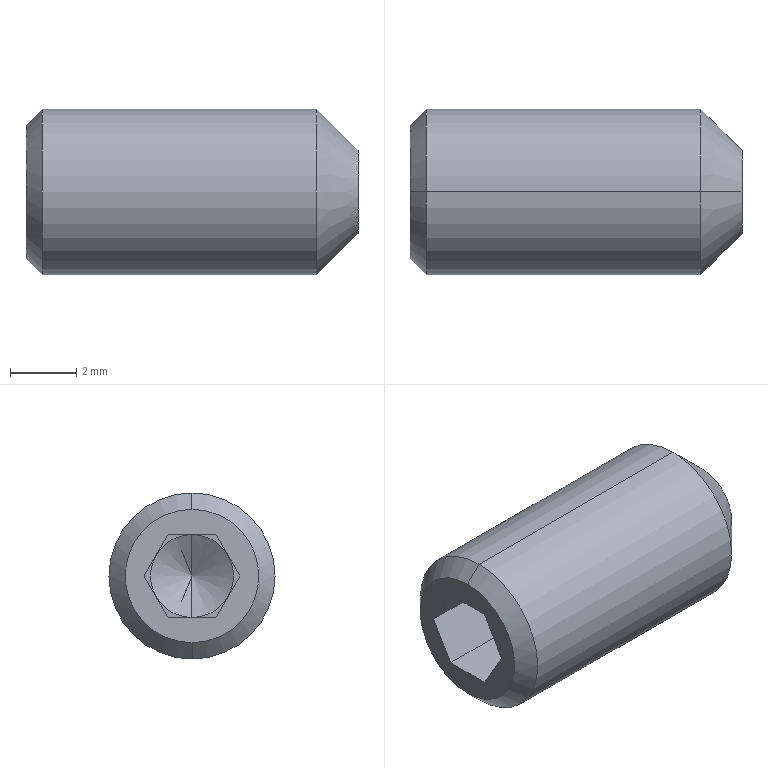Part | STEP file | 0230_301_MMSU5-10 | 1 solid | 23 faces | box 10 x 5 x 5 mm | volume 171.124 mm3 | plane 13 | cone 8 | cylinder 2 | commonest cylinder face diameters 5 x2
STEP:
#1=CARTESIAN_POINT('',(0.,0.,0.));
#2=DIRECTION('',(0.,0.,1.));
#3=DIRECTION('',(1.,0.,0.));
#4=AXIS2_PLACEMENT_3D('',#1,#2,#3);
#5=CARTESIAN_POINT('',(-4.51,0.,-2.5));
#6=VERTEX_POINT('',#5);
#7=CARTESIAN_POINT('',(-4.51,0.,2.5));
#8=VERTEX_POINT('',#7);
#9=CARTESIAN_POINT('',(-4.51,0.,0.));
#10=DIRECTION('',(1.,0.,0.));
#11=DIRECTION('',(0.,0.,-1.));
#12=AXIS2_PLACEMENT_3D('',#9,#10,#11);
#13=CIRCLE('',#12,2.5);
#14=CARTESIAN_POINT('',(-0.3797,0.,0.));
#15=DIRECTION('',(1.,0.,0.));
#16=DIRECTION('',(0.,0.,-1.));
#17=AXIS2_PLACEMENT_3D('',#14,#15,#16);
#18=CYLINDRICAL_SURFACE('',#17,2.5);
#19=CARTESIAN_POINT('',(0.,-4.13));
#20=DIRECTION('',(1.,0.));
#21=VECTOR('',#20,1.);
#22=LINE('',#19,#21);
#23=(GEOMETRIC_REPRESENTATION_CONTEXT(2)PARAMETRIC_REPRESENTATION_CONTEXT()REPRESENTATION_CONTEXT('',''));
#24=DEFINITIONAL_REPRESENTATION('',(#22),#23);
#25=PCURVE('',#18,#24);
#26=CARTESIAN_POINT('',(-4.51,0.,0.));
#27=DIRECTION('',(1.,0.,0.));
#28=DIRECTION('',(0.,0.,-1.));
#29=AXIS2_PLACEMENT_3D('',#26,#27,#28);
#30=CONICAL_SURFACE('',#29,2.5,0.7854);
#31=CARTESIAN_POINT('',(0.,0.));
#32=DIRECTION('',(1.,0.));
#33=VECTOR('',#32,1.);
#34=LINE('',#31,#33);
#35=(GEOMETRIC_REPRESENTATION_CONTEXT(2)PARAMETRIC_REPRESENTATION_CONTEXT()REPRESENTATION_CONTEXT('',''));
#36=DEFINITIONAL_REPRESENTATION('',(#34),#35);
#37=PCURVE('',#30,#36);
#38=SURFACE_CURVE('',#13,(#25,#37),.PCURVE_S1.);
#39=EDGE_CURVE('',#6,#8,#38,.T.);
#40=ORIENTED_EDGE('',*,*,#39,.T.);
#41=CARTESIAN_POINT('',(3.75,0.,2.5));
#42=VERTEX_POINT('',#41);
#43=CARTESIAN_POINT('',(-0.3797,0.,2.5));
#44=DIRECTION('',(1.,0.,0.));
#45=VECTOR('',#44,1.);
#46=LINE('',#43,#45);
#47=CARTESIAN_POINT('',(3.142,0.));
#48=DIRECTION('',(0.,1.));
#49=VECTOR('',#48,1.);
#50=LINE('',#47,#49);
#51=(GEOMETRIC_REPRESENTATION_CONTEXT(2)PARAMETRIC_REPRESENTATION_CONTEXT()REPRESENTATION_CONTEXT('',''));
#52=DEFINITIONAL_REPRESENTATION('',(#50),#51);
#53=PCURVE('',#18,#52);
#54=CARTESIAN_POINT('',(-0.3797,0.,0.));
#55=DIRECTION('',(1.,0.,0.));
#56=DIRECTION('',(0.,0.,-1.));
#57=AXIS2_PLACEMENT_3D('',#54,#55,#56);
#58=CYLINDRICAL_SURFACE('',#57,2.5);
#59=CARTESIAN_POINT('',(3.142,0.));
#60=DIRECTION('',(0.,1.));
#61=VECTOR('',#60,1.);
#62=LINE('',#59,#61);
#63=(GEOMETRIC_REPRESENTATION_CONTEXT(2)PARAMETRIC_REPRESENTATION_CONTEXT()REPRESENTATION_CONTEXT('',''));
#64=DEFINITIONAL_REPRESENTATION('',(#62),#63);
#65=PCURVE('',#58,#64);
#66=SURFACE_CURVE('',#46,(#53,#65),.PCURVE_S1.);
#67=EDGE_CURVE('',#8,#42,#66,.T.);
#68=ORIENTED_EDGE('',*,*,#67,.T.);
#69=CARTESIAN_POINT('',(3.75,0.,-2.5));
#70=VERTEX_POINT('',#69);
#71=CARTESIAN_POINT('',(3.75,0.,0.));
#72=DIRECTION('',(-1.,0.,0.));
#73=DIRECTION('',(0.,0.,-1.));
#74=AXIS2_PLACEMENT_3D('',#71,#72,#73);
#75=CIRCLE('',#74,2.5);
#76=CARTESIAN_POINT('',(6.283,4.13));
#77=DIRECTION('',(-1.,0.));
#78=VECTOR('',#77,1.);
#79=LINE('',#76,#78);
#80=(GEOMETRIC_REPRESENTATION_CONTEXT(2)PARAMETRIC_REPRESENTATION_CONTEXT()REPRESENTATION_CONTEXT('',''));
#81=DEFINITIONAL_REPRESENTATION('',(#79),#80);
#82=PCURVE('',#18,#81);
#83=CARTESIAN_POINT('',(3.75,0.,0.));
#84=DIRECTION('',(-1.,0.,0.));
#85=DIRECTION('',(0.,0.,1.));
#86=AXIS2_PLACEMENT_3D('',#83,#84,#85);
#87=CONICAL_SURFACE('',#86,2.5,0.7854);
#88=CARTESIAN_POINT('',(-3.142,0.));
#89=DIRECTION('',(1.,0.));
#90=VECTOR('',#89,1.);
#91=LINE('',#88,#90);
#92=(GEOMETRIC_REPRESENTATION_CONTEXT(2)PARAMETRIC_REPRESENTATION_CONTEXT()REPRESENTATION_CONTEXT('',''));
#93=DEFINITIONAL_REPRESENTATION('',(#91),#92);
#94=PCURVE('',#87,#93);
#95=SURFACE_CURVE('',#75,(#82,#94),.PCURVE_S1.);
#96=EDGE_CURVE('',#42,#70,#95,.T.);
#97=ORIENTED_EDGE('',*,*,#96,.T.);
#98=CARTESIAN_POINT('',(-0.3797,0.,-2.5));
#99=DIRECTION('',(1.,0.,0.));
#100=VECTOR('',#99,1.);
#101=LINE('',#98,#100);
#102=CARTESIAN_POINT('',(0.,0.));
#103=DIRECTION('',(0.,1.));
#104=VECTOR('',#103,1.);
#105=LINE('',#102,#104);
#106=(GEOMETRIC_REPRESENTATION_CONTEXT(2)PARAMETRIC_REPRESENTATION_CONTEXT()REPRESENTATION_CONTEXT('',''));
#107=DEFINITIONAL_REPRESENTATION('',(#105),#106);
#108=PCURVE('',#18,#107);
#109=CARTESIAN_POINT('',(6.283,0.));
#110=DIRECTION('',(0.,1.));
#111=VECTOR('',#110,1.);
#112=LINE('',#109,#111);
#113=(GEOMETRIC_REPRESENTATION_CONTEXT(2)PARAMETRIC_REPRESENTATION_CONTEXT()REPRESENTATION_CONTEXT('',''));
#114=DEFINITIONAL_REPRESENTATION('',(#112),#113);
#115=PCURVE('',#58,#114);
#116=SURFACE_CURVE('',#101,(#108,#115),.PCURVE_S1.);
#117=EDGE_CURVE('',#6,#70,#116,.T.);
#118=ORIENTED_EDGE('',*,*,#117,.F.);
#119=EDGE_LOOP('',(#40,#68,#97,#118));
#120=FACE_BOUND('',#119,.T.);
#121=ADVANCED_FACE('',(#120),#18,.T.);
#122=CARTESIAN_POINT('',(-5.,0.,-2.009));
#123=VERTEX_POINT('',#122);
#124=CARTESIAN_POINT('',(-5.,0.,2.009));
#125=VERTEX_POINT('',#124);
#126=CARTESIAN_POINT('',(-5.,0.,0.));
#127=DIRECTION('',(1.,0.,0.));
#128=DIRECTION('',(0.,0.,-1.));
#129=AXIS2_PLACEMENT_3D('',#126,#127,#128);
#130=CIRCLE('',#129,2.009);
#131=CARTESIAN_POINT('',(0.,-0.4905));
#132=DIRECTION('',(1.,0.));
#133=VECTOR('',#132,1.);
#134=LINE('',#131,#133);
#135=(GEOMETRIC_REPRESENTATION_CONTEXT(2)PARAMETRIC_REPRESENTATION_CONTEXT()REPRESENTATION_CONTEXT('',''));
#136=DEFINITIONAL_REPRESENTATION('',(#134),#135);
#137=PCURVE('',#30,#136);
#138=CARTESIAN_POINT('',(-5.,1.005,0.));
#139=DIRECTION('',(-1.,0.,0.));
#140=DIRECTION('',(0.,0.,1.));
#141=AXIS2_PLACEMENT_3D('',#138,#139,#140);
#142=PLANE('',#141);
#143=CARTESIAN_POINT('',(-2.009,-1.005));
#144=CARTESIAN_POINT('',(-2.009,2.476));
#145=CARTESIAN_POINT('',(1.005,0.7355));
#146=CARTESIAN_POINT('',(4.019,-1.005));
#147=CARTESIAN_POINT('',(1.005,-2.745));
#148=CARTESIAN_POINT('',(-2.009,-4.485));
#149=CARTESIAN_POINT('',(-2.009,-1.005));
#150=(BOUNDED_CURVE()B_SPLINE_CURVE(2,(#143,#144,#145,#146,#147,#148,#149),.UNSPECIFIED.,.T.,.F.)B_SPLINE_CURVE_WITH_KNOTS((1,2,2,2,2,1),(-2.094,0.,2.094,4.189,6.283,8.378),.UNSPECIFIED.)CURVE()GEOMETRIC_REPRESENTATION_ITEM()RATIONAL_B_SPLINE_CURVE((1.,0.5,1.,0.5,1.,0.5,1.))REPRESENTATION_ITEM(''));
#151=(GEOMETRIC_REPRESENTATION_CONTEXT(2)PARAMETRIC_REPRESENTATION_CONTEXT()REPRESENTATION_CONTEXT('',''));
#152=DEFINITIONAL_REPRESENTATION('',(#150),#151);
#153=PCURVE('',#142,#152);
#154=SURFACE_CURVE('',#130,(#137,#153),.PCURVE_S1.);
#155=EDGE_CURVE('',#123,#125,#154,.T.);
#156=ORIENTED_EDGE('',*,*,#155,.T.);
#157=CARTESIAN_POINT('',(-4.51,0.,2.5));
#158=DIRECTION('',(0.7071,0.,0.7071));
#159=VECTOR('',#158,1.);
#160=LINE('',#157,#159);
#161=CARTESIAN_POINT('',(3.142,0.));
#162=DIRECTION('',(0.,1.));
#163=VECTOR('',#162,1.);
#164=LINE('',#161,#163);
#165=(GEOMETRIC_REPRESENTATION_CONTEXT(2)PARAMETRIC_REPRESENTATION_CONTEXT()REPRESENTATION_CONTEXT('',''));
#166=DEFINITIONAL_REPRESENTATION('',(#164),#165);
#167=PCURVE('',#30,#166);
#168=CARTESIAN_POINT('',(-4.51,0.,0.));
#169=DIRECTION('',(1.,0.,0.));
#170=DIRECTION('',(0.,0.,-1.));
#171=AXIS2_PLACEMENT_3D('',#168,#169,#170);
#172=CONICAL_SURFACE('',#171,2.5,0.7854);
#173=CARTESIAN_POINT('',(3.142,0.));
#174=DIRECTION('',(0.,1.));
#175=VECTOR('',#174,1.);
#176=LINE('',#173,#175);
#177=(GEOMETRIC_REPRESENTATION_CONTEXT(2)PARAMETRIC_REPRESENTATION_CONTEXT()REPRESENTATION_CONTEXT('',''));
#178=DEFINITIONAL_REPRESENTATION('',(#176),#177);
#179=PCURVE('',#172,#178);
#180=SURFACE_CURVE('',#160,(#167,#179),.PCURVE_S1.);
#181=EDGE_CURVE('',#125,#8,#180,.T.);
#182=ORIENTED_EDGE('',*,*,#181,.T.);
#183=ORIENTED_EDGE('',*,*,#39,.F.);
#184=CARTESIAN_POINT('',(-4.51,0.,-2.5));
#185=DIRECTION('',(0.7071,0.,-0.7071));
#186=VECTOR('',#185,1.);
#187=LINE('',#184,#186);
#188=CARTESIAN_POINT('',(0.,0.));
#189=DIRECTION('',(0.,1.));
#190=VECTOR('',#189,1.);
#191=LINE('',#188,#190);
#192=(GEOMETRIC_REPRESENTATION_CONTEXT(2)PARAMETRIC_REPRESENTATION_CONTEXT()REPRESENTATION_CONTEXT('',''));
#193=DEFINITIONAL_REPRESENTATION('',(#191),#192);
#194=PCURVE('',#30,#193);
#195=CARTESIAN_POINT('',(6.283,0.));
#196=DIRECTION('',(0.,1.));
#197=VECTOR('',#196,1.);
#198=LINE('',#195,#197);
#199=(GEOMETRIC_REPRESENTATION_CONTEXT(2)PARAMETRIC_REPRESENTATION_CONTEXT()REPRESENTATION_CONTEXT('',''));
#200=DEFINITIONAL_REPRESENTATION('',(#198),#199);
#201=PCURVE('',#172,#200);
#202=SURFACE_CURVE('',#187,(#194,#201),.PCURVE_S1.);
#203=EDGE_CURVE('',#123,#6,#202,.T.);
#204=ORIENTED_EDGE('',*,*,#203,.F.);
#205=EDGE_LOOP('',(#156,#182,#183,#204));
#206=FACE_BOUND('',#205,.T.);
#207=ADVANCED_FACE('',(#206),#30,.T.);
#208=CARTESIAN_POINT('',(5.,0.,1.25));
#209=VERTEX_POINT('',#208);
#210=CARTESIAN_POINT('',(5.,0.,-1.25));
#211=VERTEX_POINT('',#210);
#212=CARTESIAN_POINT('',(5.,0.,0.));
#213=DIRECTION('',(-1.,0.,0.));
#214=DIRECTION('',(0.,1.,0.));
#215=AXIS2_PLACEMENT_3D('',#212,#213,#214);
#216=CIRCLE('',#215,1.25);
#217=CARTESIAN_POINT('',(-4.712,-1.25));
#218=DIRECTION('',(1.,0.));
#219=VECTOR('',#218,1.);
#220=LINE('',#217,#219);
#221=(GEOMETRIC_REPRESENTATION_CONTEXT(2)PARAMETRIC_REPRESENTATION_CONTEXT()REPRESENTATION_CONTEXT('',''));
#222=DEFINITIONAL_REPRESENTATION('',(#220),#221);
#223=PCURVE('',#87,#222);
#224=CARTESIAN_POINT('',(5.,0.,0.));
#225=DIRECTION('',(1.,0.,0.));
#226=DIRECTION('',(0.,0.,-1.));
#227=AXIS2_PLACEMENT_3D('',#224,#225,#226);
#228=CONICAL_SURFACE('',#227,1.25,1.03);
#229=CARTESIAN_POINT('',(7.854,0.));
#230=DIRECTION('',(-1.,0.));
#231=VECTOR('',#230,1.);
#232=LINE('',#229,#231);
#233=(GEOMETRIC_REPRESENTATION_CONTEXT(2)PARAMETRIC_REPRESENTATION_CONTEXT()REPRESENTATION_CONTEXT('',''));
#234=DEFINITIONAL_REPRESENTATION('',(#232),#233);
#235=PCURVE('',#228,#234);
#236=SURFACE_CURVE('',#216,(#223,#235),.PCURVE_S1.);
#237=EDGE_CURVE('',#209,#211,#236,.T.);
#238=ORIENTED_EDGE('',*,*,#237,.T.);
#239=CARTESIAN_POINT('',(3.75,0.,-2.5));
#240=DIRECTION('',(-0.7071,0.,-0.7071));
#241=VECTOR('',#240,1.);
#242=LINE('',#239,#241);
#243=CARTESIAN_POINT('',(3.142,0.));
#244=DIRECTION('',(0.,1.));
#245=VECTOR('',#244,1.);
#246=LINE('',#243,#245);
#247=(GEOMETRIC_REPRESENTATION_CONTEXT(2)PARAMETRIC_REPRESENTATION_CONTEXT()REPRESENTATION_CONTEXT('',''));
#248=DEFINITIONAL_REPRESENTATION('',(#246),#247);
#249=PCURVE('',#87,#248);
#250=CARTESIAN_POINT('',(3.75,0.,0.));
#251=DIRECTION('',(-1.,0.,0.));
#252=DIRECTION('',(0.,0.,1.));
#253=AXIS2_PLACEMENT_3D('',#250,#251,#252);
#254=CONICAL_SURFACE('',#253,2.5,0.7854);
#255=CARTESIAN_POINT('',(3.142,0.));
#256=DIRECTION('',(0.,1.));
#257=VECTOR('',#256,1.);
#258=LINE('',#255,#257);
#259=(GEOMETRIC_REPRESENTATION_CONTEXT(2)PARAMETRIC_REPRESENTATION_CONTEXT()REPRESENTATION_CONTEXT('',''));
#260=DEFINITIONAL_REPRESENTATION('',(#258),#259);
#261=PCURVE('',#254,#260);
#262=SURFACE_CURVE('',#242,(#249,#261),.PCURVE_S1.);
#263=EDGE_CURVE('',#211,#70,#262,.T.);
#264=ORIENTED_EDGE('',*,*,#263,.T.);
#265=ORIENTED_EDGE('',*,*,#96,.F.);
#266=CARTESIAN_POINT('',(3.75,0.,2.5));
#267=DIRECTION('',(-0.7071,0.,0.7071));
#268=VECTOR('',#267,1.);
#269=LINE('',#266,#268);
#270=CARTESIAN_POINT('',(0.,0.));
#271=DIRECTION('',(0.,1.));
#272=VECTOR('',#271,1.);
#273=LINE('',#270,#272);
#274=(GEOMETRIC_REPRESENTATION_CONTEXT(2)PARAMETRIC_REPRESENTATION_CONTEXT()REPRESENTATION_CONTEXT('',''));
#275=DEFINITIONAL_REPRESENTATION('',(#273),#274);
#276=PCURVE('',#87,#275);
#277=CARTESIAN_POINT('',(6.283,0.));
#278=DIRECTION('',(0.,1.));
#279=VECTOR('',#278,1.);
#280=LINE('',#277,#279);
#281=(GEOMETRIC_REPRESENTATION_CONTEXT(2)PARAMETRIC_REPRESENTATION_CONTEXT()REPRESENTATION_CONTEXT('',''));
#282=DEFINITIONAL_REPRESENTATION('',(#280),#281);
#283=PCURVE('',#254,#282);
#284=SURFACE_CURVE('',#269,(#276,#283),.PCURVE_S1.);
#285=EDGE_CURVE('',#209,#42,#284,.T.);
#286=ORIENTED_EDGE('',*,*,#285,.F.);
#287=EDGE_LOOP('',(#238,#264,#265,#286));
#288=FACE_BOUND('',#287,.T.);
#289=ADVANCED_FACE('',(#288),#87,.T.);
#290=CARTESIAN_POINT('',(5.,0.,0.));
#291=DIRECTION('',(-1.,0.,0.));
#292=DIRECTION('',(0.,1.,0.));
#293=AXIS2_PLACEMENT_3D('',#290,#291,#292);
#294=CIRCLE('',#293,1.25);
#295=CARTESIAN_POINT('',(5.,0.,0.));
#296=DIRECTION('',(1.,0.,0.));
#297=DIRECTION('',(0.,0.,-1.));
#298=AXIS2_PLACEMENT_3D('',#295,#296,#297);
#299=CONICAL_SURFACE('',#298,1.25,1.03);
#300=CARTESIAN_POINT('',(7.854,0.));
#301=DIRECTION('',(-1.,0.));
#302=VECTOR('',#301,1.);
#303=LINE('',#300,#302);
#304=(GEOMETRIC_REPRESENTATION_CONTEXT(2)PARAMETRIC_REPRESENTATION_CONTEXT()REPRESENTATION_CONTEXT('',''));
#305=DEFINITIONAL_REPRESENTATION('',(#303),#304);
#306=PCURVE('',#299,#305);
#307=CARTESIAN_POINT('',(1.571,-1.25));
#308=DIRECTION('',(1.,0.));
#309=VECTOR('',#308,1.);
#310=LINE('',#307,#309);
#311=(GEOMETRIC_REPRESENTATION_CONTEXT(2)PARAMETRIC_REPRESENTATION_CONTEXT()REPRESENTATION_CONTEXT('',''));
#312=DEFINITIONAL_REPRESENTATION('',(#310),#311);
#313=PCURVE('',#254,#312);
#314=SURFACE_CURVE('',#294,(#306,#313),.PCURVE_S1.);
#315=EDGE_CURVE('',#211,#209,#314,.T.);
#316=ORIENTED_EDGE('',*,*,#315,.T.);
#317=CARTESIAN_POINT('',(4.25,0.,0.));
#318=VERTEX_POINT('',#317);
#319=CARTESIAN_POINT('',(5.,0.,1.25));
#320=DIRECTION('',(0.5145,0.,0.8575));
#321=VECTOR('',#320,1.);
#322=LINE('',#319,#321);
#323=CARTESIAN_POINT('',(3.142,0.));
#324=DIRECTION('',(0.,1.));
#325=VECTOR('',#324,1.);
#326=LINE('',#323,#325);
#327=(GEOMETRIC_REPRESENTATION_CONTEXT(2)PARAMETRIC_REPRESENTATION_CONTEXT()REPRESENTATION_CONTEXT('',''));
#328=DEFINITIONAL_REPRESENTATION('',(#326),#327);
#329=PCURVE('',#299,#328);
#330=CARTESIAN_POINT('',(3.142,0.));
#331=DIRECTION('',(0.,1.));
#332=VECTOR('',#331,1.);
#333=LINE('',#330,#332);
#334=(GEOMETRIC_REPRESENTATION_CONTEXT(2)PARAMETRIC_REPRESENTATION_CONTEXT()REPRESENTATION_CONTEXT('',''));
#335=DEFINITIONAL_REPRESENTATION('',(#333),#334);
#336=PCURVE('',#228,#335);
#337=SURFACE_CURVE('',#322,(#329,#336),.PCURVE_S1.);
#338=EDGE_CURVE('',#318,#209,#337,.T.);
#339=ORIENTED_EDGE('',*,*,#338,.F.);
#340=CARTESIAN_POINT('',(5.,0.,-1.25));
#341=DIRECTION('',(0.5145,0.,-0.8575));
#342=VECTOR('',#341,1.);
#343=LINE('',#340,#342);
#344=CARTESIAN_POINT('',(6.283,0.));
#345=DIRECTION('',(0.,1.));
#346=VECTOR('',#345,1.);
#347=LINE('',#344,#346);
#348=(GEOMETRIC_REPRESENTATION_CONTEXT(2)PARAMETRIC_REPRESENTATION_CONTEXT()REPRESENTATION_CONTEXT('',''));
#349=DEFINITIONAL_REPRESENTATION('',(#347),#348);
#350=PCURVE('',#299,#349);
#351=CARTESIAN_POINT('',(0.,0.));
#352=DIRECTION('',(0.,1.));
#353=VECTOR('',#352,1.);
#354=LINE('',#351,#353);
#355=(GEOMETRIC_REPRESENTATION_CONTEXT(2)PARAMETRIC_REPRESENTATION_CONTEXT()REPRESENTATION_CONTEXT('',''));
#356=DEFINITIONAL_REPRESENTATION('',(#354),#355);
#357=PCURVE('',#228,#356);
#358=SURFACE_CURVE('',#343,(#350,#357),.PCURVE_S1.);
#359=EDGE_CURVE('',#318,#211,#358,.T.);
#360=ORIENTED_EDGE('',*,*,#359,.T.);
#361=EDGE_LOOP('',(#316,#339,#360));
#362=FACE_BOUND('',#361,.F.);
#363=ADVANCED_FACE('',(#362),#299,.F.);
#364=CARTESIAN_POINT('',(-3.,0.,1.25));
#365=VERTEX_POINT('',#364);
#366=CARTESIAN_POINT('',(-3.,-1.083,0.625));
#367=VERTEX_POINT('',#366);
#368=CARTESIAN_POINT('',(-3.,0.,0.));
#369=DIRECTION('',(1.,0.,0.));
#370=DIRECTION('',(0.,0.,1.));
#371=AXIS2_PLACEMENT_3D('',#368,#369,#370);
#372=CIRCLE('',#371,1.25);
#373=CARTESIAN_POINT('',(-3.,0.,0.));
#374=DIRECTION('',(-1.,0.,0.));
#375=DIRECTION('',(0.,0.,1.));
#376=AXIS2_PLACEMENT_3D('',#373,#374,#375);
#377=CONICAL_SURFACE('',#376,1.25,1.047);
#378=CARTESIAN_POINT('',(6.283,0.));
#379=DIRECTION('',(-1.,0.));
#380=VECTOR('',#379,1.);
#381=LINE('',#378,#380);
#382=(GEOMETRIC_REPRESENTATION_CONTEXT(2)PARAMETRIC_REPRESENTATION_CONTEXT()REPRESENTATION_CONTEXT('',''));
#383=DEFINITIONAL_REPRESENTATION('',(#381),#382);
#384=PCURVE('',#377,#383);
#385=CARTESIAN_POINT('',(-3.,0.,0.));
#386=DIRECTION('',(1.,0.,0.));
#387=DIRECTION('',(0.,0.,-1.));
#388=AXIS2_PLACEMENT_3D('',#385,#386,#387);
#389=PLANE('',#388);
#390=CARTESIAN_POINT('',(0.,0.));
#391=DIRECTION('',(-1.,0.));
#392=AXIS2_PLACEMENT_2D('',#390,#391);
#393=CIRCLE('',#392,1.25);
#394=(GEOMETRIC_REPRESENTATION_CONTEXT(2)PARAMETRIC_REPRESENTATION_CONTEXT()REPRESENTATION_CONTEXT('',''));
#395=DEFINITIONAL_REPRESENTATION('',(#393),#394);
#396=PCURVE('',#389,#395);
#397=SURFACE_CURVE('',#372,(#384,#396),.PCURVE_S1.);
#398=EDGE_CURVE('',#365,#367,#397,.T.);
#399=ORIENTED_EDGE('',*,*,#398,.T.);
#400=CARTESIAN_POINT('',(-3.,-1.083,-0.625));
#401=VERTEX_POINT('',#400);
#402=CARTESIAN_POINT('',(-3.,0.,0.));
#403=DIRECTION('',(1.,0.,0.));
#404=DIRECTION('',(0.,0.,1.));
#405=AXIS2_PLACEMENT_3D('',#402,#403,#404);
#406=CIRCLE('',#405,1.25);
#407=CARTESIAN_POINT('',(6.283,0.));
#408=DIRECTION('',(-1.,0.));
#409=VECTOR('',#408,1.);
#410=LINE('',#407,#409);
#411=(GEOMETRIC_REPRESENTATION_CONTEXT(2)PARAMETRIC_REPRESENTATION_CONTEXT()REPRESENTATION_CONTEXT('',''));
#412=DEFINITIONAL_REPRESENTATION('',(#410),#411);
#413=PCURVE('',#377,#412);
#414=CARTESIAN_POINT('',(-3.,0.,0.));
#415=DIRECTION('',(1.,0.,0.));
#416=DIRECTION('',(0.,0.,-1.));
#417=AXIS2_PLACEMENT_3D('',#414,#415,#416);
#418=PLANE('',#417);
#419=CARTESIAN_POINT('',(0.,0.));
#420=DIRECTION('',(-1.,0.));
#421=AXIS2_PLACEMENT_2D('',#419,#420);
#422=CIRCLE('',#421,1.25);
#423=(GEOMETRIC_REPRESENTATION_CONTEXT(2)PARAMETRIC_REPRESENTATION_CONTEXT()REPRESENTATION_CONTEXT('',''));
#424=DEFINITIONAL_REPRESENTATION('',(#422),#423);
#425=PCURVE('',#418,#424);
#426=SURFACE_CURVE('',#406,(#413,#425),.PCURVE_S1.);
#427=EDGE_CURVE('',#367,#401,#426,.T.);
#428=ORIENTED_EDGE('',*,*,#427,.T.);
#429=CARTESIAN_POINT('',(-3.,0.,-1.25));
#430=VERTEX_POINT('',#429);
#431=CARTESIAN_POINT('',(-3.,0.,0.));
#432=DIRECTION('',(-1.,0.,0.));
#433=DIRECTION('',(0.,0.,1.));
#434=AXIS2_PLACEMENT_3D('',#431,#432,#433);
#435=CIRCLE('',#434,1.25);
#436=CARTESIAN_POINT('',(0.,0.));
#437=DIRECTION('',(1.,0.));
#438=VECTOR('',#437,1.);
#439=LINE('',#436,#438);
#440=(GEOMETRIC_REPRESENTATION_CONTEXT(2)PARAMETRIC_REPRESENTATION_CONTEXT()REPRESENTATION_CONTEXT('',''));
#441=DEFINITIONAL_REPRESENTATION('',(#439),#440);
#442=PCURVE('',#377,#441);
#443=CARTESIAN_POINT('',(-3.,0.,0.));
#444=DIRECTION('',(1.,0.,0.));
#445=DIRECTION('',(0.,0.,-1.));
#446=AXIS2_PLACEMENT_3D('',#443,#444,#445);
#447=PLANE('',#446);
#448=CARTESIAN_POINT('',(-1.25,0.));
#449=CARTESIAN_POINT('',(-1.25,2.165));
#450=CARTESIAN_POINT('',(0.625,1.083));
#451=CARTESIAN_POINT('',(2.5,0.));
#452=CARTESIAN_POINT('',(0.625,-1.083));
#453=CARTESIAN_POINT('',(-1.25,-2.165));
#454=CARTESIAN_POINT('',(-1.25,0.));
#455=(BOUNDED_CURVE()B_SPLINE_CURVE(2,(#448,#449,#450,#451,#452,#453,#454),.UNSPECIFIED.,.T.,.F.)B_SPLINE_CURVE_WITH_KNOTS((1,2,2,2,2,1),(-2.094,0.,2.094,4.189,6.283,8.378),.UNSPECIFIED.)CURVE()GEOMETRIC_REPRESENTATION_ITEM()RATIONAL_B_SPLINE_CURVE((1.,0.5,1.,0.5,1.,0.5,1.))REPRESENTATION_ITEM(''));
#456=(GEOMETRIC_REPRESENTATION_CONTEXT(2)PARAMETRIC_REPRESENTATION_CONTEXT()REPRESENTATION_CONTEXT('',''));
#457=DEFINITIONAL_REPRESENTATION('',(#455),#456);
#458=PCURVE('',#447,#457);
#459=SURFACE_CURVE('',#435,(#442,#458),.PCURVE_S1.);
#460=EDGE_CURVE('',#430,#401,#459,.T.);
#461=ORIENTED_EDGE('',*,*,#460,.F.);
#462=CARTESIAN_POINT('',(-2.278,0.,0.));
#463=VERTEX_POINT('',#462);
#464=CARTESIAN_POINT('',(-3.,0.,-1.25));
#465=DIRECTION('',(-0.5,0.,-0.866));
#466=VECTOR('',#465,1.);
#467=LINE('',#464,#466);
#468=CARTESIAN_POINT('',(3.142,0.));
#469=DIRECTION('',(0.,1.));
#470=VECTOR('',#469,1.);
#471=LINE('',#468,#470);
#472=(GEOMETRIC_REPRESENTATION_CONTEXT(2)PARAMETRIC_REPRESENTATION_CONTEXT()REPRESENTATION_CONTEXT('',''));
#473=DEFINITIONAL_REPRESENTATION('',(#471),#472);
#474=PCURVE('',#377,#473);
#475=CARTESIAN_POINT('',(-3.,0.,0.));
#476=DIRECTION('',(-1.,0.,0.));
#477=DIRECTION('',(0.,0.,1.));
#478=AXIS2_PLACEMENT_3D('',#475,#476,#477);
#479=CONICAL_SURFACE('',#478,1.25,1.047);
#480=CARTESIAN_POINT('',(3.142,0.));
#481=DIRECTION('',(0.,1.));
#482=VECTOR('',#481,1.);
#483=LINE('',#480,#482);
#484=(GEOMETRIC_REPRESENTATION_CONTEXT(2)PARAMETRIC_REPRESENTATION_CONTEXT()REPRESENTATION_CONTEXT('',''));
#485=DEFINITIONAL_REPRESENTATION('',(#483),#484);
#486=PCURVE('',#479,#485);
#487=SURFACE_CURVE('',#467,(#474,#486),.PCURVE_S1.);
#488=EDGE_CURVE('',#463,#430,#487,.T.);
#489=ORIENTED_EDGE('',*,*,#488,.F.);
#490=CARTESIAN_POINT('',(-3.,0.,1.25));
#491=DIRECTION('',(-0.5,0.,0.866));
#492=VECTOR('',#491,1.);
#493=LINE('',#490,#492);
#494=CARTESIAN_POINT('',(6.283,0.));
#495=DIRECTION('',(0.,1.));
#496=VECTOR('',#495,1.);
#497=LINE('',#494,#496);
#498=(GEOMETRIC_REPRESENTATION_CONTEXT(2)PARAMETRIC_REPRESENTATION_CONTEXT()REPRESENTATION_CONTEXT('',''));
#499=DEFINITIONAL_REPRESENTATION('',(#497),#498);
#500=PCURVE('',#377,#499);
#501=CARTESIAN_POINT('',(0.,0.));
#502=DIRECTION('',(0.,1.));
#503=VECTOR('',#502,1.);
#504=LINE('',#501,#503);
#505=(GEOMETRIC_REPRESENTATION_CONTEXT(2)PARAMETRIC_REPRESENTATION_CONTEXT()REPRESENTATION_CONTEXT('',''));
#506=DEFINITIONAL_REPRESENTATION('',(#504),#505);
#507=PCURVE('',#479,#506);
#508=SURFACE_CURVE('',#493,(#500,#507),.PCURVE_S1.);
#509=EDGE_CURVE('',#463,#365,#508,.T.);
#510=ORIENTED_EDGE('',*,*,#509,.T.);
#511=EDGE_LOOP('',(#399,#428,#461,#489,#510));
#512=FACE_BOUND('',#511,.F.);
#513=ADVANCED_FACE('',(#512),#377,.F.);
#514=ORIENTED_EDGE('',*,*,#67,.F.);
#515=CARTESIAN_POINT('',(-4.51,0.,0.));
#516=DIRECTION('',(1.,0.,0.));
#517=DIRECTION('',(0.,0.,-1.));
#518=AXIS2_PLACEMENT_3D('',#515,#516,#517);
#519=CIRCLE('',#518,2.5);
#520=CARTESIAN_POINT('',(0.,-4.13));
#521=DIRECTION('',(1.,0.));
#522=VECTOR('',#521,1.);
#523=LINE('',#520,#522);
#524=(GEOMETRIC_REPRESENTATION_CONTEXT(2)PARAMETRIC_REPRESENTATION_CONTEXT()REPRESENTATION_CONTEXT('',''));
#525=DEFINITIONAL_REPRESENTATION('',(#523),#524);
#526=PCURVE('',#58,#525);
#527=CARTESIAN_POINT('',(0.,0.));
#528=DIRECTION('',(1.,0.));
#529=VECTOR('',#528,1.);
#530=LINE('',#527,#529);
#531=(GEOMETRIC_REPRESENTATION_CONTEXT(2)PARAMETRIC_REPRESENTATION_CONTEXT()REPRESENTATION_CONTEXT('',''));
#532=DEFINITIONAL_REPRESENTATION('',(#530),#531);
#533=PCURVE('',#172,#532);
#534=SURFACE_CURVE('',#519,(#526,#533),.PCURVE_S1.);
#535=EDGE_CURVE('',#8,#6,#534,.T.);
#536=ORIENTED_EDGE('',*,*,#535,.T.);
#537=ORIENTED_EDGE('',*,*,#117,.T.);
#538=CARTESIAN_POINT('',(3.75,0.,0.));
#539=DIRECTION('',(-1.,0.,0.));
#540=DIRECTION('',(0.,0.,-1.));
#541=AXIS2_PLACEMENT_3D('',#538,#539,#540);
#542=CIRCLE('',#541,2.5);
#543=CARTESIAN_POINT('',(6.283,4.13));
#544=DIRECTION('',(-1.,0.));
#545=VECTOR('',#544,1.);
#546=LINE('',#543,#545);
#547=(GEOMETRIC_REPRESENTATION_CONTEXT(2)PARAMETRIC_REPRESENTATION_CONTEXT()REPRESENTATION_CONTEXT('',''));
#548=DEFINITIONAL_REPRESENTATION('',(#546),#547);
#549=PCURVE('',#58,#548);
#550=CARTESIAN_POINT('',(3.142,0.));
#551=DIRECTION('',(1.,0.));
#552=VECTOR('',#551,1.);
#553=LINE('',#550,#552);
#554=(GEOMETRIC_REPRESENTATION_CONTEXT(2)PARAMETRIC_REPRESENTATION_CONTEXT()REPRESENTATION_CONTEXT('',''));
#555=DEFINITIONAL_REPRESENTATION('',(#553),#554);
#556=PCURVE('',#254,#555);
#557=SURFACE_CURVE('',#542,(#549,#556),.PCURVE_S1.);
#558=EDGE_CURVE('',#70,#42,#557,.T.);
#559=ORIENTED_EDGE('',*,*,#558,.T.);
#560=EDGE_LOOP('',(#514,#536,#537,#559));
#561=FACE_BOUND('',#560,.T.);
#562=ADVANCED_FACE('',(#561),#58,.T.);
#563=ORIENTED_EDGE('',*,*,#181,.F.);
#564=CARTESIAN_POINT('',(-5.,0.,0.));
#565=DIRECTION('',(1.,0.,0.));
#566=DIRECTION('',(0.,0.,-1.));
#567=AXIS2_PLACEMENT_3D('',#564,#565,#566);
#568=CIRCLE('',#567,2.009);
#569=CARTESIAN_POINT('',(0.,-0.4905));
#570=DIRECTION('',(1.,0.));
#571=VECTOR('',#570,1.);
#572=LINE('',#569,#571);
#573=(GEOMETRIC_REPRESENTATION_CONTEXT(2)PARAMETRIC_REPRESENTATION_CONTEXT()REPRESENTATION_CONTEXT('',''));
#574=DEFINITIONAL_REPRESENTATION('',(#572),#573);
#575=PCURVE('',#172,#574);
#576=CARTESIAN_POINT('',(-2.009,-1.005));
#577=CARTESIAN_POINT('',(-2.009,2.476));
#578=CARTESIAN_POINT('',(1.005,0.7355));
#579=CARTESIAN_POINT('',(4.019,-1.005));
#580=CARTESIAN_POINT('',(1.005,-2.745));
#581=CARTESIAN_POINT('',(-2.009,-4.485));
#582=CARTESIAN_POINT('',(-2.009,-1.005));
#583=(BOUNDED_CURVE()B_SPLINE_CURVE(2,(#576,#577,#578,#579,#580,#581,#582),.UNSPECIFIED.,.T.,.F.)B_SPLINE_CURVE_WITH_KNOTS((1,2,2,2,2,1),(-2.094,0.,2.094,4.189,6.283,8.378),.UNSPECIFIED.)CURVE()GEOMETRIC_REPRESENTATION_ITEM()RATIONAL_B_SPLINE_CURVE((1.,0.5,1.,0.5,1.,0.5,1.))REPRESENTATION_ITEM(''));
#584=(GEOMETRIC_REPRESENTATION_CONTEXT(2)PARAMETRIC_REPRESENTATION_CONTEXT()REPRESENTATION_CONTEXT('',''));
#585=DEFINITIONAL_REPRESENTATION('',(#583),#584);
#586=PCURVE('',#142,#585);
#587=SURFACE_CURVE('',#568,(#575,#586),.PCURVE_S1.);
#588=EDGE_CURVE('',#125,#123,#587,.T.);
#589=ORIENTED_EDGE('',*,*,#588,.T.);
#590=ORIENTED_EDGE('',*,*,#203,.T.);
#591=ORIENTED_EDGE('',*,*,#535,.F.);
#592=EDGE_LOOP('',(#563,#589,#590,#591));
#593=FACE_BOUND('',#592,.T.);
#594=ADVANCED_FACE('',(#593),#172,.T.);
#595=ORIENTED_EDGE('',*,*,#263,.F.);
#596=ORIENTED_EDGE('',*,*,#315,.T.);
#597=ORIENTED_EDGE('',*,*,#285,.T.);
#598=ORIENTED_EDGE('',*,*,#558,.F.);
#599=EDGE_LOOP('',(#595,#596,#597,#598));
#600=FACE_BOUND('',#599,.T.);
#601=ADVANCED_FACE('',(#600),#254,.T.);
#602=ORIENTED_EDGE('',*,*,#155,.F.);
#603=ORIENTED_EDGE('',*,*,#588,.F.);
#604=EDGE_LOOP('',(#602,#603));
#605=FACE_BOUND('',#604,.T.);
#606=CARTESIAN_POINT('',(-5.,-0.7217,-1.25));
#607=VERTEX_POINT('',#606);
#608=CARTESIAN_POINT('',(-5.,0.7217,-1.25));
#609=VERTEX_POINT('',#608);
#610=CARTESIAN_POINT('',(-5.,0.7217,-1.25));
#611=DIRECTION('',(0.,1.,0.));
#612=VECTOR('',#611,1.);
#613=LINE('',#610,#612);
#614=CARTESIAN_POINT('',(-1.25,-0.2831));
#615=DIRECTION('',(0.,1.));
#616=VECTOR('',#615,1.);
#617=LINE('',#614,#616);
#618=(GEOMETRIC_REPRESENTATION_CONTEXT(2)PARAMETRIC_REPRESENTATION_CONTEXT()REPRESENTATION_CONTEXT('',''));
#619=DEFINITIONAL_REPRESENTATION('',(#617),#618);
#620=PCURVE('',#142,#619);
#621=CARTESIAN_POINT('',(-5.,0.7217,-1.25));
#622=DIRECTION('',(0.,0.,-1.));
#623=DIRECTION('',(-1.,0.,0.));
#624=AXIS2_PLACEMENT_3D('',#621,#622,#623);
#625=PLANE('',#624);
#626=CARTESIAN_POINT('',(0.,0.));
#627=DIRECTION('',(0.,1.));
#628=VECTOR('',#627,1.);
#629=LINE('',#626,#628);
#630=(GEOMETRIC_REPRESENTATION_CONTEXT(2)PARAMETRIC_REPRESENTATION_CONTEXT()REPRESENTATION_CONTEXT('',''));
#631=DEFINITIONAL_REPRESENTATION('',(#629),#630);
#632=PCURVE('',#625,#631);
#633=SURFACE_CURVE('',#613,(#620,#632),.PCURVE_S1.);
#634=EDGE_CURVE('',#607,#609,#633,.T.);
#635=ORIENTED_EDGE('',*,*,#634,.T.);
#636=CARTESIAN_POINT('',(-5.,1.443,0.));
#637=VERTEX_POINT('',#636);
#638=CARTESIAN_POINT('',(-5.,0.7217,-1.25));
#639=DIRECTION('',(0.,0.5,0.866));
#640=VECTOR('',#639,1.);
#641=LINE('',#638,#640);
#642=CARTESIAN_POINT('',(-1.25,-0.2831));
#643=DIRECTION('',(0.866,0.5));
#644=VECTOR('',#643,1.);
#645=LINE('',#642,#644);
#646=(GEOMETRIC_REPRESENTATION_CONTEXT(2)PARAMETRIC_REPRESENTATION_CONTEXT()REPRESENTATION_CONTEXT('',''));
#647=DEFINITIONAL_REPRESENTATION('',(#645),#646);
#648=PCURVE('',#142,#647);
#649=CARTESIAN_POINT('',(-5.,1.443,0.));
#650=DIRECTION('',(0.,0.866,-0.5));
#651=DIRECTION('',(0.,0.5,0.866));
#652=AXIS2_PLACEMENT_3D('',#649,#650,#651);
#653=PLANE('',#652);
#654=CARTESIAN_POINT('',(-1.443,0.));
#655=DIRECTION('',(1.,0.));
#656=VECTOR('',#655,1.);
#657=LINE('',#654,#656);
#658=(GEOMETRIC_REPRESENTATION_CONTEXT(2)PARAMETRIC_REPRESENTATION_CONTEXT()REPRESENTATION_CONTEXT('',''));
#659=DEFINITIONAL_REPRESENTATION('',(#657),#658);
#660=PCURVE('',#653,#659);
#661=SURFACE_CURVE('',#641,(#648,#660),.PCURVE_S1.);
#662=EDGE_CURVE('',#609,#637,#661,.T.);
#663=ORIENTED_EDGE('',*,*,#662,.T.);
#664=CARTESIAN_POINT('',(-5.,0.7217,1.25));
#665=VERTEX_POINT('',#664);
#666=CARTESIAN_POINT('',(-5.,0.7217,1.25));
#667=DIRECTION('',(0.,-0.5,0.866));
#668=VECTOR('',#667,1.);
#669=LINE('',#666,#668);
#670=CARTESIAN_POINT('',(1.25,-0.2831));
#671=DIRECTION('',(0.866,-0.5));
#672=VECTOR('',#671,1.);
#673=LINE('',#670,#672);
#674=(GEOMETRIC_REPRESENTATION_CONTEXT(2)PARAMETRIC_REPRESENTATION_CONTEXT()REPRESENTATION_CONTEXT('',''));
#675=DEFINITIONAL_REPRESENTATION('',(#673),#674);
#676=PCURVE('',#142,#675);
#677=CARTESIAN_POINT('',(-5.,0.7217,1.25));
#678=DIRECTION('',(0.,0.866,0.5));
#679=DIRECTION('',(0.,-0.5,0.866));
#680=AXIS2_PLACEMENT_3D('',#677,#678,#679);
#681=PLANE('',#680);
#682=CARTESIAN_POINT('',(0.,0.));
#683=DIRECTION('',(1.,0.));
#684=VECTOR('',#683,1.);
#685=LINE('',#682,#684);
#686=(GEOMETRIC_REPRESENTATION_CONTEXT(2)PARAMETRIC_REPRESENTATION_CONTEXT()REPRESENTATION_CONTEXT('',''));
#687=DEFINITIONAL_REPRESENTATION('',(#685),#686);
#688=PCURVE('',#681,#687);
#689=SURFACE_CURVE('',#669,(#676,#688),.PCURVE_S1.);
#690=EDGE_CURVE('',#637,#665,#689,.T.);
#691=ORIENTED_EDGE('',*,*,#690,.T.);
#692=CARTESIAN_POINT('',(-5.,-0.7217,1.25));
#693=VERTEX_POINT('',#692);
#694=CARTESIAN_POINT('',(-5.,-0.7217,1.25));
#695=DIRECTION('',(0.,-1.,0.));
#696=VECTOR('',#695,1.);
#697=LINE('',#694,#696);
#698=CARTESIAN_POINT('',(1.25,-1.726));
#699=DIRECTION('',(0.,-1.));
#700=VECTOR('',#699,1.);
#701=LINE('',#698,#700);
#702=(GEOMETRIC_REPRESENTATION_CONTEXT(2)PARAMETRIC_REPRESENTATION_CONTEXT()REPRESENTATION_CONTEXT('',''));
#703=DEFINITIONAL_REPRESENTATION('',(#701),#702);
#704=PCURVE('',#142,#703);
#705=CARTESIAN_POINT('',(-5.,-0.7217,1.25));
#706=DIRECTION('',(0.,0.,1.));
#707=DIRECTION('',(1.,0.,0.));
#708=AXIS2_PLACEMENT_3D('',#705,#706,#707);
#709=PLANE('',#708);
#710=CARTESIAN_POINT('',(0.,0.));
#711=DIRECTION('',(0.,-1.));
#712=VECTOR('',#711,1.);
#713=LINE('',#710,#712);
#714=(GEOMETRIC_REPRESENTATION_CONTEXT(2)PARAMETRIC_REPRESENTATION_CONTEXT()REPRESENTATION_CONTEXT('',''));
#715=DEFINITIONAL_REPRESENTATION('',(#713),#714);
#716=PCURVE('',#709,#715);
#717=SURFACE_CURVE('',#697,(#704,#716),.PCURVE_S1.);
#718=EDGE_CURVE('',#665,#693,#717,.T.);
#719=ORIENTED_EDGE('',*,*,#718,.T.);
#720=CARTESIAN_POINT('',(-5.,-1.443,0.));
#721=VERTEX_POINT('',#720);
#722=CARTESIAN_POINT('',(-5.,-1.443,0.));
#723=DIRECTION('',(0.,-0.5,-0.866));
#724=VECTOR('',#723,1.);
#725=LINE('',#722,#724);
#726=CARTESIAN_POINT('',(0.,-2.448));
#727=DIRECTION('',(-0.866,-0.5));
#728=VECTOR('',#727,1.);
#729=LINE('',#726,#728);
#730=(GEOMETRIC_REPRESENTATION_CONTEXT(2)PARAMETRIC_REPRESENTATION_CONTEXT()REPRESENTATION_CONTEXT('',''));
#731=DEFINITIONAL_REPRESENTATION('',(#729),#730);
#732=PCURVE('',#142,#731);
#733=CARTESIAN_POINT('',(-5.,-1.443,0.));
#734=DIRECTION('',(0.,-0.866,0.5));
#735=DIRECTION('',(0.,-0.5,-0.866));
#736=AXIS2_PLACEMENT_3D('',#733,#734,#735);
#737=PLANE('',#736);
#738=CARTESIAN_POINT('',(0.,0.));
#739=DIRECTION('',(1.,0.));
#740=VECTOR('',#739,1.);
#741=LINE('',#738,#740);
#742=(GEOMETRIC_REPRESENTATION_CONTEXT(2)PARAMETRIC_REPRESENTATION_CONTEXT()REPRESENTATION_CONTEXT('',''));
#743=DEFINITIONAL_REPRESENTATION('',(#741),#742);
#744=PCURVE('',#737,#743);
#745=SURFACE_CURVE('',#725,(#732,#744),.PCURVE_S1.);
#746=EDGE_CURVE('',#693,#721,#745,.T.);
#747=ORIENTED_EDGE('',*,*,#746,.T.);
#748=CARTESIAN_POINT('',(-5.,-0.7217,-1.25));
#749=DIRECTION('',(0.,0.5,-0.866));
#750=VECTOR('',#749,1.);
#751=LINE('',#748,#750);
#752=CARTESIAN_POINT('',(-1.25,-1.726));
#753=DIRECTION('',(-0.866,0.5));
#754=VECTOR('',#753,1.);
#755=LINE('',#752,#754);
#756=(GEOMETRIC_REPRESENTATION_CONTEXT(2)PARAMETRIC_REPRESENTATION_CONTEXT()REPRESENTATION_CONTEXT('',''));
#757=DEFINITIONAL_REPRESENTATION('',(#755),#756);
#758=PCURVE('',#142,#757);
#759=CARTESIAN_POINT('',(-5.,-0.7217,-1.25));
#760=DIRECTION('',(0.,-0.866,-0.5));
#761=DIRECTION('',(0.,0.5,-0.866));
#762=AXIS2_PLACEMENT_3D('',#759,#760,#761);
#763=PLANE('',#762);
#764=CARTESIAN_POINT('',(0.,0.));
#765=DIRECTION('',(1.,0.));
#766=VECTOR('',#765,1.);
#767=LINE('',#764,#766);
#768=(GEOMETRIC_REPRESENTATION_CONTEXT(2)PARAMETRIC_REPRESENTATION_CONTEXT()REPRESENTATION_CONTEXT('',''));
#769=DEFINITIONAL_REPRESENTATION('',(#767),#768);
#770=PCURVE('',#763,#769);
#771=SURFACE_CURVE('',#751,(#758,#770),.PCURVE_S1.);
#772=EDGE_CURVE('',#721,#607,#771,.T.);
#773=ORIENTED_EDGE('',*,*,#772,.T.);
#774=EDGE_LOOP('',(#635,#663,#691,#719,#747,#773));
#775=FACE_BOUND('',#774,.T.);
#776=ADVANCED_FACE('',(#605,#775),#142,.T.);
#777=ORIENTED_EDGE('',*,*,#237,.T.);
#778=ORIENTED_EDGE('',*,*,#359,.F.);
#779=ORIENTED_EDGE('',*,*,#338,.T.);
#780=EDGE_LOOP('',(#777,#778,#779));
#781=FACE_BOUND('',#780,.F.);
#782=ADVANCED_FACE('',(#781),#228,.F.);
#783=CARTESIAN_POINT('',(-3.,1.443,0.));
#784=VERTEX_POINT('',#783);
#785=CARTESIAN_POINT('',(-5.,1.443,0.));
#786=DIRECTION('',(1.,0.,0.));
#787=VECTOR('',#786,1.);
#788=LINE('',#785,#787);
#789=CARTESIAN_POINT('',(0.,0.));
#790=DIRECTION('',(0.,1.));
#791=VECTOR('',#790,1.);
#792=LINE('',#789,#791);
#793=(GEOMETRIC_REPRESENTATION_CONTEXT(2)PARAMETRIC_REPRESENTATION_CONTEXT()REPRESENTATION_CONTEXT('',''));
#794=DEFINITIONAL_REPRESENTATION('',(#792),#793);
#795=PCURVE('',#653,#794);
#796=CARTESIAN_POINT('',(-1.443,0.));
#797=DIRECTION('',(0.,1.));
#798=VECTOR('',#797,1.);
#799=LINE('',#796,#798);
#800=(GEOMETRIC_REPRESENTATION_CONTEXT(2)PARAMETRIC_REPRESENTATION_CONTEXT()REPRESENTATION_CONTEXT('',''));
#801=DEFINITIONAL_REPRESENTATION('',(#799),#800);
#802=PCURVE('',#681,#801);
#803=SURFACE_CURVE('',#788,(#795,#802),.PCURVE_S1.);
#804=EDGE_CURVE('',#637,#784,#803,.T.);
#805=ORIENTED_EDGE('',*,*,#804,.F.);
#806=ORIENTED_EDGE('',*,*,#662,.F.);
#807=CARTESIAN_POINT('',(-3.,0.7217,-1.25));
#808=VERTEX_POINT('',#807);
#809=CARTESIAN_POINT('',(-5.,0.7217,-1.25));
#810=DIRECTION('',(-1.,0.,0.));
#811=VECTOR('',#810,1.);
#812=LINE('',#809,#811);
#813=CARTESIAN_POINT('',(-1.443,0.));
#814=DIRECTION('',(0.,-1.));
#815=VECTOR('',#814,1.);
#816=LINE('',#813,#815);
#817=(GEOMETRIC_REPRESENTATION_CONTEXT(2)PARAMETRIC_REPRESENTATION_CONTEXT()REPRESENTATION_CONTEXT('',''));
#818=DEFINITIONAL_REPRESENTATION('',(#816),#817);
#819=PCURVE('',#653,#818);
#820=CARTESIAN_POINT('',(0.,0.));
#821=DIRECTION('',(1.,0.));
#822=VECTOR('',#821,1.);
#823=LINE('',#820,#822);
#824=(GEOMETRIC_REPRESENTATION_CONTEXT(2)PARAMETRIC_REPRESENTATION_CONTEXT()REPRESENTATION_CONTEXT('',''));
#825=DEFINITIONAL_REPRESENTATION('',(#823),#824);
#826=PCURVE('',#625,#825);
#827=SURFACE_CURVE('',#812,(#819,#826),.PCURVE_S1.);
#828=EDGE_CURVE('',#808,#609,#827,.T.);
#829=ORIENTED_EDGE('',*,*,#828,.F.);
#830=CARTESIAN_POINT('',(-3.,1.083,-0.625));
#831=VERTEX_POINT('',#830);
#832=CARTESIAN_POINT('',(-3.,1.443,0.));
#833=DIRECTION('',(0.,-0.5,-0.866));
#834=VECTOR('',#833,1.);
#835=LINE('',#832,#834);
#836=CARTESIAN_POINT('',(0.,2.));
#837=DIRECTION('',(-1.,0.));
#838=VECTOR('',#837,1.);
#839=LINE('',#836,#838);
#840=(GEOMETRIC_REPRESENTATION_CONTEXT(2)PARAMETRIC_REPRESENTATION_CONTEXT()REPRESENTATION_CONTEXT('',''));
#841=DEFINITIONAL_REPRESENTATION('',(#839),#840);
#842=PCURVE('',#653,#841);
#843=CARTESIAN_POINT('',(-3.,0.,0.));
#844=DIRECTION('',(1.,0.,0.));
#845=DIRECTION('',(0.,0.,-1.));
#846=AXIS2_PLACEMENT_3D('',#843,#844,#845);
#847=PLANE('',#846);
#848=CARTESIAN_POINT('',(0.,1.443));
#849=DIRECTION('',(0.866,-0.5));
#850=VECTOR('',#849,1.);
#851=LINE('',#848,#850);
#852=(GEOMETRIC_REPRESENTATION_CONTEXT(2)PARAMETRIC_REPRESENTATION_CONTEXT()REPRESENTATION_CONTEXT('',''));
#853=DEFINITIONAL_REPRESENTATION('',(#851),#852);
#854=PCURVE('',#847,#853);
#855=SURFACE_CURVE('',#835,(#842,#854),.PCURVE_S1.);
#856=EDGE_CURVE('',#831,#808,#855,.T.);
#857=ORIENTED_EDGE('',*,*,#856,.F.);
#858=CARTESIAN_POINT('',(-3.,1.443,0.));
#859=DIRECTION('',(0.,-0.5,-0.866));
#860=VECTOR('',#859,1.);
#861=LINE('',#858,#860);
#862=CARTESIAN_POINT('',(0.,2.));
#863=DIRECTION('',(-1.,0.));
#864=VECTOR('',#863,1.);
#865=LINE('',#862,#864);
#866=(GEOMETRIC_REPRESENTATION_CONTEXT(2)PARAMETRIC_REPRESENTATION_CONTEXT()REPRESENTATION_CONTEXT('',''));
#867=DEFINITIONAL_REPRESENTATION('',(#865),#866);
#868=PCURVE('',#653,#867);
#869=CARTESIAN_POINT('',(-3.,0.,0.));
#870=DIRECTION('',(1.,0.,0.));
#871=DIRECTION('',(0.,0.,-1.));
#872=AXIS2_PLACEMENT_3D('',#869,#870,#871);
#873=PLANE('',#872);
#874=CARTESIAN_POINT('',(0.,1.443));
#875=DIRECTION('',(0.866,-0.5));
#876=VECTOR('',#875,1.);
#877=LINE('',#874,#876);
#878=(GEOMETRIC_REPRESENTATION_CONTEXT(2)PARAMETRIC_REPRESENTATION_CONTEXT()REPRESENTATION_CONTEXT('',''));
#879=DEFINITIONAL_REPRESENTATION('',(#877),#878);
#880=PCURVE('',#873,#879);
#881=SURFACE_CURVE('',#861,(#868,#880),.PCURVE_S1.);
#882=EDGE_CURVE('',#784,#831,#881,.T.);
#883=ORIENTED_EDGE('',*,*,#882,.F.);
#884=EDGE_LOOP('',(#805,#806,#829,#857,#883));
#885=FACE_BOUND('',#884,.T.);
#886=ADVANCED_FACE('',(#885),#653,.F.);
#887=CARTESIAN_POINT('',(-3.,1.083,0.625));
#888=VERTEX_POINT('',#887);
#889=CARTESIAN_POINT('',(-3.,0.,0.));
#890=DIRECTION('',(1.,0.,0.));
#891=DIRECTION('',(0.,0.,1.));
#892=AXIS2_PLACEMENT_3D('',#889,#890,#891);
#893=CIRCLE('',#892,1.25);
#894=CARTESIAN_POINT('',(0.,0.));
#895=DIRECTION('',(-1.,0.));
#896=AXIS2_PLACEMENT_2D('',#894,#895);
#897=CIRCLE('',#896,1.25);
#898=(GEOMETRIC_REPRESENTATION_CONTEXT(2)PARAMETRIC_REPRESENTATION_CONTEXT()REPRESENTATION_CONTEXT('',''));
#899=DEFINITIONAL_REPRESENTATION('',(#897),#898);
#900=PCURVE('',#873,#899);
#901=CARTESIAN_POINT('',(6.283,0.));
#902=DIRECTION('',(-1.,0.));
#903=VECTOR('',#902,1.);
#904=LINE('',#901,#903);
#905=(GEOMETRIC_REPRESENTATION_CONTEXT(2)PARAMETRIC_REPRESENTATION_CONTEXT()REPRESENTATION_CONTEXT('',''));
#906=DEFINITIONAL_REPRESENTATION('',(#904),#905);
#907=PCURVE('',#479,#906);
#908=SURFACE_CURVE('',#893,(#900,#907),.PCURVE_S1.);
#909=EDGE_CURVE('',#831,#888,#908,.T.);
#910=ORIENTED_EDGE('',*,*,#909,.T.);
#911=CARTESIAN_POINT('',(-3.,1.443,0.));
#912=DIRECTION('',(0.,-0.5,0.866));
#913=VECTOR('',#912,1.);
#914=LINE('',#911,#913);
#915=CARTESIAN_POINT('',(0.,1.443));
#916=DIRECTION('',(-0.866,-0.5));
#917=VECTOR('',#916,1.);
#918=LINE('',#915,#917);
#919=(GEOMETRIC_REPRESENTATION_CONTEXT(2)PARAMETRIC_REPRESENTATION_CONTEXT()REPRESENTATION_CONTEXT('',''));
#920=DEFINITIONAL_REPRESENTATION('',(#918),#919);
#921=PCURVE('',#873,#920);
#922=CARTESIAN_POINT('',(-1.443,2.));
#923=DIRECTION('',(1.,0.));
#924=VECTOR('',#923,1.);
#925=LINE('',#922,#924);
#926=(GEOMETRIC_REPRESENTATION_CONTEXT(2)PARAMETRIC_REPRESENTATION_CONTEXT()REPRESENTATION_CONTEXT('',''));
#927=DEFINITIONAL_REPRESENTATION('',(#925),#926);
#928=PCURVE('',#681,#927);
#929=SURFACE_CURVE('',#914,(#921,#928),.PCURVE_S1.);
#930=EDGE_CURVE('',#784,#888,#929,.T.);
#931=ORIENTED_EDGE('',*,*,#930,.F.);
#932=ORIENTED_EDGE('',*,*,#882,.T.);
#933=EDGE_LOOP('',(#910,#931,#932));
#934=FACE_BOUND('',#933,.T.);
#935=ADVANCED_FACE('',(#934),#873,.F.);
#936=CARTESIAN_POINT('',(-3.,0.7217,1.25));
#937=VERTEX_POINT('',#936);
#938=CARTESIAN_POINT('',(-5.,0.7217,1.25));
#939=DIRECTION('',(1.,0.,0.));
#940=VECTOR('',#939,1.);
#941=LINE('',#938,#940);
#942=CARTESIAN_POINT('',(0.,0.));
#943=DIRECTION('',(0.,1.));
#944=VECTOR('',#943,1.);
#945=LINE('',#942,#944);
#946=(GEOMETRIC_REPRESENTATION_CONTEXT(2)PARAMETRIC_REPRESENTATION_CONTEXT()REPRESENTATION_CONTEXT('',''));
#947=DEFINITIONAL_REPRESENTATION('',(#945),#946);
#948=PCURVE('',#681,#947);
#949=CARTESIAN_POINT('',(0.,1.443));
#950=DIRECTION('',(1.,0.));
#951=VECTOR('',#950,1.);
#952=LINE('',#949,#951);
#953=(GEOMETRIC_REPRESENTATION_CONTEXT(2)PARAMETRIC_REPRESENTATION_CONTEXT()REPRESENTATION_CONTEXT('',''));
#954=DEFINITIONAL_REPRESENTATION('',(#952),#953);
#955=PCURVE('',#709,#954);
#956=SURFACE_CURVE('',#941,(#948,#955),.PCURVE_S1.);
#957=EDGE_CURVE('',#665,#937,#956,.T.);
#958=ORIENTED_EDGE('',*,*,#957,.F.);
#959=ORIENTED_EDGE('',*,*,#690,.F.);
#960=ORIENTED_EDGE('',*,*,#804,.T.);
#961=ORIENTED_EDGE('',*,*,#930,.T.);
#962=CARTESIAN_POINT('',(-3.,0.7217,1.25));
#963=DIRECTION('',(0.,0.5,-0.866));
#964=VECTOR('',#963,1.);
#965=LINE('',#962,#964);
#966=CARTESIAN_POINT('',(0.,2.));
#967=DIRECTION('',(-1.,0.));
#968=VECTOR('',#967,1.);
#969=LINE('',#966,#968);
#970=(GEOMETRIC_REPRESENTATION_CONTEXT(2)PARAMETRIC_REPRESENTATION_CONTEXT()REPRESENTATION_CONTEXT('',''));
#971=DEFINITIONAL_REPRESENTATION('',(#969),#970);
#972=PCURVE('',#681,#971);
#973=CARTESIAN_POINT('',(-3.,0.,0.));
#974=DIRECTION('',(1.,0.,0.));
#975=DIRECTION('',(0.,0.,-1.));
#976=AXIS2_PLACEMENT_3D('',#973,#974,#975);
#977=PLANE('',#976);
#978=CARTESIAN_POINT('',(-1.25,0.7217));
#979=DIRECTION('',(0.866,0.5));
#980=VECTOR('',#979,1.);
#981=LINE('',#978,#980);
#982=(GEOMETRIC_REPRESENTATION_CONTEXT(2)PARAMETRIC_REPRESENTATION_CONTEXT()REPRESENTATION_CONTEXT('',''));
#983=DEFINITIONAL_REPRESENTATION('',(#981),#982);
#984=PCURVE('',#977,#983);
#985=SURFACE_CURVE('',#965,(#972,#984),.PCURVE_S1.);
#986=EDGE_CURVE('',#937,#888,#985,.T.);
#987=ORIENTED_EDGE('',*,*,#986,.F.);
#988=EDGE_LOOP('',(#958,#959,#960,#961,#987));
#989=FACE_BOUND('',#988,.T.);
#990=ADVANCED_FACE('',(#989),#681,.F.);
#991=ORIENTED_EDGE('',*,*,#828,.T.);
#992=ORIENTED_EDGE('',*,*,#634,.F.);
#993=CARTESIAN_POINT('',(-3.,-0.7217,-1.25));
#994=VERTEX_POINT('',#993);
#995=CARTESIAN_POINT('',(-5.,-0.7217,-1.25));
#996=DIRECTION('',(-1.,0.,0.));
#997=VECTOR('',#996,1.);
#998=LINE('',#995,#997);
#999=CARTESIAN_POINT('',(0.,-1.443));
#1000=DIRECTION('',(1.,0.));
#1001=VECTOR('',#1000,1.);
#1002=LINE('',#999,#1001);
#1003=(GEOMETRIC_REPRESENTATION_CONTEXT(2)PARAMETRIC_REPRESENTATION_CONTEXT()REPRESENTATION_CONTEXT('',''));
#1004=DEFINITIONAL_REPRESENTATION('',(#1002),#1003);
#1005=PCURVE('',#625,#1004);
#1006=CARTESIAN_POINT('',(0.,0.));
#1007=DIRECTION('',(0.,-1.));
#1008=VECTOR('',#1007,1.);
#1009=LINE('',#1006,#1008);
#1010=(GEOMETRIC_REPRESENTATION_CONTEXT(2)PARAMETRIC_REPRESENTATION_CONTEXT()REPRESENTATION_CONTEXT('',''));
#1011=DEFINITIONAL_REPRESENTATION('',(#1009),#1010);
#1012=PCURVE('',#763,#1011);
#1013=SURFACE_CURVE('',#998,(#1005,#1012),.PCURVE_S1.);
#1014=EDGE_CURVE('',#994,#607,#1013,.T.);
#1015=ORIENTED_EDGE('',*,*,#1014,.F.);
#1016=CARTESIAN_POINT('',(-3.,0.7217,-1.25));
#1017=DIRECTION('',(0.,-1.,0.));
#1018=VECTOR('',#1017,1.);
#1019=LINE('',#1016,#1018);
#1020=CARTESIAN_POINT('',(-2.,0.));
#1021=DIRECTION('',(0.,-1.));
#1022=VECTOR('',#1021,1.);
#1023=LINE('',#1020,#1022);
#1024=(GEOMETRIC_REPRESENTATION_CONTEXT(2)PARAMETRIC_REPRESENTATION_CONTEXT()REPRESENTATION_CONTEXT('',''));
#1025=DEFINITIONAL_REPRESENTATION('',(#1023),#1024);
#1026=PCURVE('',#625,#1025);
#1027=CARTESIAN_POINT('',(1.25,0.7217));
#1028=DIRECTION('',(0.,-1.));
#1029=VECTOR('',#1028,1.);
#1030=LINE('',#1027,#1029);
#1031=(GEOMETRIC_REPRESENTATION_CONTEXT(2)PARAMETRIC_REPRESENTATION_CONTEXT()REPRESENTATION_CONTEXT('',''));
#1032=DEFINITIONAL_REPRESENTATION('',(#1030),#1031);
#1033=PCURVE('',#447,#1032);
#1034=SURFACE_CURVE('',#1019,(#1026,#1033),.PCURVE_S1.);
#1035=EDGE_CURVE('',#430,#994,#1034,.T.);
#1036=ORIENTED_EDGE('',*,*,#1035,.F.);
#1037=CARTESIAN_POINT('',(-3.,0.7217,-1.25));
#1038=DIRECTION('',(0.,-1.,0.));
#1039=VECTOR('',#1038,1.);
#1040=LINE('',#1037,#1039);
#1041=CARTESIAN_POINT('',(-2.,0.));
#1042=DIRECTION('',(0.,-1.));
#1043=VECTOR('',#1042,1.);
#1044=LINE('',#1041,#1043);
#1045=(GEOMETRIC_REPRESENTATION_CONTEXT(2)PARAMETRIC_REPRESENTATION_CONTEXT()REPRESENTATION_CONTEXT('',''));
#1046=DEFINITIONAL_REPRESENTATION('',(#1044),#1045);
#1047=PCURVE('',#625,#1046);
#1048=CARTESIAN_POINT('',(1.25,0.7217));
#1049=DIRECTION('',(0.,-1.));
#1050=VECTOR('',#1049,1.);
#1051=LINE('',#1048,#1050);
#1052=(GEOMETRIC_REPRESENTATION_CONTEXT(2)PARAMETRIC_REPRESENTATION_CONTEXT()REPRESENTATION_CONTEXT('',''));
#1053=DEFINITIONAL_REPRESENTATION('',(#1051),#1052);
#1054=PCURVE('',#847,#1053);
#1055=SURFACE_CURVE('',#1040,(#1047,#1054),.PCURVE_S1.);
#1056=EDGE_CURVE('',#808,#430,#1055,.T.);
#1057=ORIENTED_EDGE('',*,*,#1056,.F.);
#1058=EDGE_LOOP('',(#991,#992,#1015,#1036,#1057));
#1059=FACE_BOUND('',#1058,.T.);
#1060=ADVANCED_FACE('',(#1059),#625,.F.);
#1061=ORIENTED_EDGE('',*,*,#856,.T.);
#1062=ORIENTED_EDGE('',*,*,#1056,.T.);
#1063=CARTESIAN_POINT('',(-3.,0.,0.));
#1064=DIRECTION('',(-1.,0.,0.));
#1065=DIRECTION('',(0.,0.,1.));
#1066=AXIS2_PLACEMENT_3D('',#1063,#1064,#1065);
#1067=CIRCLE('',#1066,1.25);
#1068=CARTESIAN_POINT('',(-1.25,0.));
#1069=CARTESIAN_POINT('',(-1.25,2.165));
#1070=CARTESIAN_POINT('',(0.625,1.083));
#1071=CARTESIAN_POINT('',(2.5,0.));
#1072=CARTESIAN_POINT('',(0.625,-1.083));
#1073=CARTESIAN_POINT('',(-1.25,-2.165));
#1074=CARTESIAN_POINT('',(-1.25,0.));
#1075=(BOUNDED_CURVE()B_SPLINE_CURVE(2,(#1068,#1069,#1070,#1071,#1072,#1073,#1074),.UNSPECIFIED.,.T.,.F.)B_SPLINE_CURVE_WITH_KNOTS((1,2,2,2,2,1),(-2.094,0.,2.094,4.189,6.283,8.378),.UNSPECIFIED.)CURVE()GEOMETRIC_REPRESENTATION_ITEM()RATIONAL_B_SPLINE_CURVE((1.,0.5,1.,0.5,1.,0.5,1.))REPRESENTATION_ITEM(''));
#1076=(GEOMETRIC_REPRESENTATION_CONTEXT(2)PARAMETRIC_REPRESENTATION_CONTEXT()REPRESENTATION_CONTEXT('',''));
#1077=DEFINITIONAL_REPRESENTATION('',(#1075),#1076);
#1078=PCURVE('',#847,#1077);
#1079=CARTESIAN_POINT('',(0.,0.));
#1080=DIRECTION('',(1.,0.));
#1081=VECTOR('',#1080,1.);
#1082=LINE('',#1079,#1081);
#1083=(GEOMETRIC_REPRESENTATION_CONTEXT(2)PARAMETRIC_REPRESENTATION_CONTEXT()REPRESENTATION_CONTEXT('',''));
#1084=DEFINITIONAL_REPRESENTATION('',(#1082),#1083);
#1085=PCURVE('',#479,#1084);
#1086=SURFACE_CURVE('',#1067,(#1078,#1085),.PCURVE_S1.);
#1087=EDGE_CURVE('',#831,#430,#1086,.T.);
#1088=ORIENTED_EDGE('',*,*,#1087,.F.);
#1089=EDGE_LOOP('',(#1061,#1062,#1088));
#1090=FACE_BOUND('',#1089,.T.);
#1091=ADVANCED_FACE('',(#1090),#847,.F.);
#1092=CARTESIAN_POINT('',(-3.,0.,1.25));
#1093=DIRECTION('',(0.,-1.,0.));
#1094=VECTOR('',#1093,1.);
#1095=LINE('',#1092,#1094);
#1096=CARTESIAN_POINT('',(-1.25,0.));
#1097=DIRECTION('',(0.,-1.));
#1098=VECTOR('',#1097,1.);
#1099=LINE('',#1096,#1098);
#1100=(GEOMETRIC_REPRESENTATION_CONTEXT(2)PARAMETRIC_REPRESENTATION_CONTEXT()REPRESENTATION_CONTEXT('',''));
#1101=DEFINITIONAL_REPRESENTATION('',(#1099),#1100);
#1102=PCURVE('',#977,#1101);
#1103=CARTESIAN_POINT('',(2.,0.7217));
#1104=DIRECTION('',(0.,-1.));
#1105=VECTOR('',#1104,1.);
#1106=LINE('',#1103,#1105);
#1107=(GEOMETRIC_REPRESENTATION_CONTEXT(2)PARAMETRIC_REPRESENTATION_CONTEXT()REPRESENTATION_CONTEXT('',''));
#1108=DEFINITIONAL_REPRESENTATION('',(#1106),#1107);
#1109=PCURVE('',#709,#1108);
#1110=SURFACE_CURVE('',#1095,(#1102,#1109),.PCURVE_S1.);
#1111=EDGE_CURVE('',#937,#365,#1110,.T.);
#1112=ORIENTED_EDGE('',*,*,#1111,.F.);
#1113=ORIENTED_EDGE('',*,*,#986,.T.);
#1114=CARTESIAN_POINT('',(-3.,0.,0.));
#1115=DIRECTION('',(-1.,0.,0.));
#1116=DIRECTION('',(0.,0.,1.));
#1117=AXIS2_PLACEMENT_3D('',#1114,#1115,#1116);
#1118=CIRCLE('',#1117,1.25);
#1119=CARTESIAN_POINT('',(-1.25,0.));
#1120=CARTESIAN_POINT('',(-1.25,2.165));
#1121=CARTESIAN_POINT('',(0.625,1.083));
#1122=CARTESIAN_POINT('',(2.5,0.));
#1123=CARTESIAN_POINT('',(0.625,-1.083));
#1124=CARTESIAN_POINT('',(-1.25,-2.165));
#1125=CARTESIAN_POINT('',(-1.25,0.));
#1126=(BOUNDED_CURVE()B_SPLINE_CURVE(2,(#1119,#1120,#1121,#1122,#1123,#1124,#1125),.UNSPECIFIED.,.T.,.F.)B_SPLINE_CURVE_WITH_KNOTS((1,2,2,2,2,1),(-2.094,0.,2.094,4.189,6.283,8.378),.UNSPECIFIED.)CURVE()GEOMETRIC_REPRESENTATION_ITEM()RATIONAL_B_SPLINE_CURVE((1.,0.5,1.,0.5,1.,0.5,1.))REPRESENTATION_ITEM(''));
#1127=(GEOMETRIC_REPRESENTATION_CONTEXT(2)PARAMETRIC_REPRESENTATION_CONTEXT()REPRESENTATION_CONTEXT('',''));
#1128=DEFINITIONAL_REPRESENTATION('',(#1126),#1127);
#1129=PCURVE('',#977,#1128);
#1130=CARTESIAN_POINT('',(0.,0.));
#1131=DIRECTION('',(1.,0.));
#1132=VECTOR('',#1131,1.);
#1133=LINE('',#1130,#1132);
#1134=(GEOMETRIC_REPRESENTATION_CONTEXT(2)PARAMETRIC_REPRESENTATION_CONTEXT()REPRESENTATION_CONTEXT('',''));
#1135=DEFINITIONAL_REPRESENTATION('',(#1133),#1134);
#1136=PCURVE('',#479,#1135);
#1137=SURFACE_CURVE('',#1118,(#1129,#1136),.PCURVE_S1.);
#1138=EDGE_CURVE('',#365,#888,#1137,.T.);
#1139=ORIENTED_EDGE('',*,*,#1138,.F.);
#1140=EDGE_LOOP('',(#1112,#1113,#1139));
#1141=FACE_BOUND('',#1140,.T.);
#1142=ADVANCED_FACE('',(#1141),#977,.F.);
#1143=CARTESIAN_POINT('',(-3.,-0.7217,1.25));
#1144=VERTEX_POINT('',#1143);
#1145=CARTESIAN_POINT('',(-5.,-0.7217,1.25));
#1146=DIRECTION('',(1.,0.,0.));
#1147=VECTOR('',#1146,1.);
#1148=LINE('',#1145,#1147);
#1149=CARTESIAN_POINT('',(0.,0.));
#1150=DIRECTION('',(1.,0.));
#1151=VECTOR('',#1150,1.);
#1152=LINE('',#1149,#1151);
#1153=(GEOMETRIC_REPRESENTATION_CONTEXT(2)PARAMETRIC_REPRESENTATION_CONTEXT()REPRESENTATION_CONTEXT('',''));
#1154=DEFINITIONAL_REPRESENTATION('',(#1152),#1153);
#1155=PCURVE('',#709,#1154);
#1156=CARTESIAN_POINT('',(-1.443,0.));
#1157=DIRECTION('',(0.,1.));
#1158=VECTOR('',#1157,1.);
#1159=LINE('',#1156,#1158);
#1160=(GEOMETRIC_REPRESENTATION_CONTEXT(2)PARAMETRIC_REPRESENTATION_CONTEXT()REPRESENTATION_CONTEXT('',''));
#1161=DEFINITIONAL_REPRESENTATION('',(#1159),#1160);
#1162=PCURVE('',#737,#1161);
#1163=SURFACE_CURVE('',#1148,(#1155,#1162),.PCURVE_S1.);
#1164=EDGE_CURVE('',#693,#1144,#1163,.T.);
#1165=ORIENTED_EDGE('',*,*,#1164,.F.);
#1166=ORIENTED_EDGE('',*,*,#718,.F.);
#1167=ORIENTED_EDGE('',*,*,#957,.T.);
#1168=ORIENTED_EDGE('',*,*,#1111,.T.);
#1169=CARTESIAN_POINT('',(-3.,-0.7217,1.25));
#1170=DIRECTION('',(0.,1.,0.));
#1171=VECTOR('',#1170,1.);
#1172=LINE('',#1169,#1171);
#1173=CARTESIAN_POINT('',(2.,0.));
#1174=DIRECTION('',(0.,1.));
#1175=VECTOR('',#1174,1.);
#1176=LINE('',#1173,#1175);
#1177=(GEOMETRIC_REPRESENTATION_CONTEXT(2)PARAMETRIC_REPRESENTATION_CONTEXT()REPRESENTATION_CONTEXT('',''));
#1178=DEFINITIONAL_REPRESENTATION('',(#1176),#1177);
#1179=PCURVE('',#709,#1178);
#1180=CARTESIAN_POINT('',(-1.25,-0.7217));
#1181=DIRECTION('',(0.,1.));
#1182=VECTOR('',#1181,1.);
#1183=LINE('',#1180,#1182);
#1184=(GEOMETRIC_REPRESENTATION_CONTEXT(2)PARAMETRIC_REPRESENTATION_CONTEXT()REPRESENTATION_CONTEXT('',''));
#1185=DEFINITIONAL_REPRESENTATION('',(#1183),#1184);
#1186=PCURVE('',#389,#1185);
#1187=SURFACE_CURVE('',#1172,(#1179,#1186),.PCURVE_S1.);
#1188=EDGE_CURVE('',#1144,#365,#1187,.T.);
#1189=ORIENTED_EDGE('',*,*,#1188,.F.);
#1190=EDGE_LOOP('',(#1165,#1166,#1167,#1168,#1189));
#1191=FACE_BOUND('',#1190,.T.);
#1192=ADVANCED_FACE('',(#1191),#709,.F.);
#1193=ORIENTED_EDGE('',*,*,#1014,.T.);
#1194=ORIENTED_EDGE('',*,*,#772,.F.);
#1195=CARTESIAN_POINT('',(-3.,-1.443,0.));
#1196=VERTEX_POINT('',#1195);
#1197=CARTESIAN_POINT('',(-5.,-1.443,0.));
#1198=DIRECTION('',(-1.,0.,0.));
#1199=VECTOR('',#1198,1.);
#1200=LINE('',#1197,#1199);
#1201=CARTESIAN_POINT('',(-1.443,0.));
#1202=DIRECTION('',(0.,-1.));
#1203=VECTOR('',#1202,1.);
#1204=LINE('',#1201,#1203);
#1205=(GEOMETRIC_REPRESENTATION_CONTEXT(2)PARAMETRIC_REPRESENTATION_CONTEXT()REPRESENTATION_CONTEXT('',''));
#1206=DEFINITIONAL_REPRESENTATION('',(#1204),#1205);
#1207=PCURVE('',#763,#1206);
#1208=CARTESIAN_POINT('',(0.,0.));
#1209=DIRECTION('',(0.,-1.));
#1210=VECTOR('',#1209,1.);
#1211=LINE('',#1208,#1210);
#1212=(GEOMETRIC_REPRESENTATION_CONTEXT(2)PARAMETRIC_REPRESENTATION_CONTEXT()REPRESENTATION_CONTEXT('',''));
#1213=DEFINITIONAL_REPRESENTATION('',(#1211),#1212);
#1214=PCURVE('',#737,#1213);
#1215=SURFACE_CURVE('',#1200,(#1207,#1214),.PCURVE_S1.);
#1216=EDGE_CURVE('',#1196,#721,#1215,.T.);
#1217=ORIENTED_EDGE('',*,*,#1216,.F.);
#1218=CARTESIAN_POINT('',(-3.,-0.7217,-1.25));
#1219=DIRECTION('',(0.,-0.5,0.866));
#1220=VECTOR('',#1219,1.);
#1221=LINE('',#1218,#1220);
#1222=CARTESIAN_POINT('',(0.,2.));
#1223=DIRECTION('',(-1.,0.));
#1224=VECTOR('',#1223,1.);
#1225=LINE('',#1222,#1224);
#1226=(GEOMETRIC_REPRESENTATION_CONTEXT(2)PARAMETRIC_REPRESENTATION_CONTEXT()REPRESENTATION_CONTEXT('',''));
#1227=DEFINITIONAL_REPRESENTATION('',(#1225),#1226);
#1228=PCURVE('',#763,#1227);
#1229=CARTESIAN_POINT('',(1.25,-0.7217));
#1230=DIRECTION('',(-0.866,-0.5));
#1231=VECTOR('',#1230,1.);
#1232=LINE('',#1229,#1231);
#1233=(GEOMETRIC_REPRESENTATION_CONTEXT(2)PARAMETRIC_REPRESENTATION_CONTEXT()REPRESENTATION_CONTEXT('',''));
#1234=DEFINITIONAL_REPRESENTATION('',(#1232),#1233);
#1235=PCURVE('',#418,#1234);
#1236=SURFACE_CURVE('',#1221,(#1228,#1235),.PCURVE_S1.);
#1237=EDGE_CURVE('',#401,#1196,#1236,.T.);
#1238=ORIENTED_EDGE('',*,*,#1237,.F.);
#1239=CARTESIAN_POINT('',(-3.,-0.7217,-1.25));
#1240=DIRECTION('',(0.,-0.5,0.866));
#1241=VECTOR('',#1240,1.);
#1242=LINE('',#1239,#1241);
#1243=CARTESIAN_POINT('',(0.,2.));
#1244=DIRECTION('',(-1.,0.));
#1245=VECTOR('',#1244,1.);
#1246=LINE('',#1243,#1245);
#1247=(GEOMETRIC_REPRESENTATION_CONTEXT(2)PARAMETRIC_REPRESENTATION_CONTEXT()REPRESENTATION_CONTEXT('',''));
#1248=DEFINITIONAL_REPRESENTATION('',(#1246),#1247);
#1249=PCURVE('',#763,#1248);
#1250=CARTESIAN_POINT('',(1.25,-0.7217));
#1251=DIRECTION('',(-0.866,-0.5));
#1252=VECTOR('',#1251,1.);
#1253=LINE('',#1250,#1252);
#1254=(GEOMETRIC_REPRESENTATION_CONTEXT(2)PARAMETRIC_REPRESENTATION_CONTEXT()REPRESENTATION_CONTEXT('',''));
#1255=DEFINITIONAL_REPRESENTATION('',(#1253),#1254);
#1256=PCURVE('',#447,#1255);
#1257=SURFACE_CURVE('',#1242,(#1249,#1256),.PCURVE_S1.);
#1258=EDGE_CURVE('',#994,#401,#1257,.T.);
#1259=ORIENTED_EDGE('',*,*,#1258,.F.);
#1260=EDGE_LOOP('',(#1193,#1194,#1217,#1238,#1259));
#1261=FACE_BOUND('',#1260,.T.);
#1262=ADVANCED_FACE('',(#1261),#763,.F.);
#1263=ORIENTED_EDGE('',*,*,#1035,.T.);
#1264=ORIENTED_EDGE('',*,*,#1258,.T.);
#1265=ORIENTED_EDGE('',*,*,#460,.F.);
#1266=EDGE_LOOP('',(#1263,#1264,#1265));
#1267=FACE_BOUND('',#1266,.T.);
#1268=ADVANCED_FACE('',(#1267),#447,.F.);
#1269=ORIENTED_EDGE('',*,*,#1087,.F.);
#1270=ORIENTED_EDGE('',*,*,#909,.T.);
#1271=ORIENTED_EDGE('',*,*,#1138,.F.);
#1272=ORIENTED_EDGE('',*,*,#509,.F.);
#1273=ORIENTED_EDGE('',*,*,#488,.T.);
#1274=EDGE_LOOP('',(#1269,#1270,#1271,#1272,#1273));
#1275=FACE_BOUND('',#1274,.F.);
#1276=ADVANCED_FACE('',(#1275),#479,.F.);
#1277=CARTESIAN_POINT('',(-3.,-0.7217,1.25));
#1278=DIRECTION('',(0.,-0.5,-0.866));
#1279=VECTOR('',#1278,1.);
#1280=LINE('',#1277,#1279);
#1281=CARTESIAN_POINT('',(-1.25,-0.7217));
#1282=DIRECTION('',(0.866,-0.5));
#1283=VECTOR('',#1282,1.);
#1284=LINE('',#1281,#1283);
#1285=(GEOMETRIC_REPRESENTATION_CONTEXT(2)PARAMETRIC_REPRESENTATION_CONTEXT()REPRESENTATION_CONTEXT('',''));
#1286=DEFINITIONAL_REPRESENTATION('',(#1284),#1285);
#1287=PCURVE('',#389,#1286);
#1288=CARTESIAN_POINT('',(-1.443,2.));
#1289=DIRECTION('',(1.,0.));
#1290=VECTOR('',#1289,1.);
#1291=LINE('',#1288,#1290);
#1292=(GEOMETRIC_REPRESENTATION_CONTEXT(2)PARAMETRIC_REPRESENTATION_CONTEXT()REPRESENTATION_CONTEXT('',''));
#1293=DEFINITIONAL_REPRESENTATION('',(#1291),#1292);
#1294=PCURVE('',#737,#1293);
#1295=SURFACE_CURVE('',#1280,(#1287,#1294),.PCURVE_S1.);
#1296=EDGE_CURVE('',#1144,#367,#1295,.T.);
#1297=ORIENTED_EDGE('',*,*,#1296,.F.);
#1298=ORIENTED_EDGE('',*,*,#1188,.T.);
#1299=ORIENTED_EDGE('',*,*,#398,.T.);
#1300=EDGE_LOOP('',(#1297,#1298,#1299));
#1301=FACE_BOUND('',#1300,.T.);
#1302=ADVANCED_FACE('',(#1301),#389,.F.);
#1303=ORIENTED_EDGE('',*,*,#1216,.T.);
#1304=ORIENTED_EDGE('',*,*,#746,.F.);
#1305=ORIENTED_EDGE('',*,*,#1164,.T.);
#1306=ORIENTED_EDGE('',*,*,#1296,.T.);
#1307=CARTESIAN_POINT('',(-3.,-1.443,0.));
#1308=DIRECTION('',(0.,0.5,0.866));
#1309=VECTOR('',#1308,1.);
#1310=LINE('',#1307,#1309);
#1311=CARTESIAN_POINT('',(0.,2.));
#1312=DIRECTION('',(-1.,0.));
#1313=VECTOR('',#1312,1.);
#1314=LINE('',#1311,#1313);
#1315=(GEOMETRIC_REPRESENTATION_CONTEXT(2)PARAMETRIC_REPRESENTATION_CONTEXT()REPRESENTATION_CONTEXT('',''));
#1316=DEFINITIONAL_REPRESENTATION('',(#1314),#1315);
#1317=PCURVE('',#737,#1316);
#1318=CARTESIAN_POINT('',(0.,-1.443));
#1319=DIRECTION('',(-0.866,0.5));
#1320=VECTOR('',#1319,1.);
#1321=LINE('',#1318,#1320);
#1322=(GEOMETRIC_REPRESENTATION_CONTEXT(2)PARAMETRIC_REPRESENTATION_CONTEXT()REPRESENTATION_CONTEXT('',''));
#1323=DEFINITIONAL_REPRESENTATION('',(#1321),#1322);
#1324=PCURVE('',#418,#1323);
#1325=SURFACE_CURVE('',#1310,(#1317,#1324),.PCURVE_S1.);
#1326=EDGE_CURVE('',#1196,#367,#1325,.T.);
#1327=ORIENTED_EDGE('',*,*,#1326,.F.);
#1328=EDGE_LOOP('',(#1303,#1304,#1305,#1306,#1327));
#1329=FACE_BOUND('',#1328,.T.);
#1330=ADVANCED_FACE('',(#1329),#737,.F.);
#1331=ORIENTED_EDGE('',*,*,#427,.T.);
#1332=ORIENTED_EDGE('',*,*,#1237,.T.);
#1333=ORIENTED_EDGE('',*,*,#1326,.T.);
#1334=EDGE_LOOP('',(#1331,#1332,#1333));
#1335=FACE_BOUND('',#1334,.T.);
#1336=ADVANCED_FACE('',(#1335),#418,.F.);
#1337=CLOSED_SHELL('',(#121,#207,#289,#363,#513,#562,#594,#601,#776,#782,#886,#935,#990,#1060,#1091,#1142,#1192,#1262,#1268,#1276,#1302,#1330,#1336));
#1338=MANIFOLD_SOLID_BREP('',#1337);
#1339=(LENGTH_UNIT()NAMED_UNIT(*)SI_UNIT(.MILLI.,.METRE.));
#1340=UNCERTAINTY_MEASURE_WITH_UNIT(LENGTH_MEASURE(0.0000001),#1339,'','');
#1341=(NAMED_UNIT(*)PLANE_ANGLE_UNIT()SI_UNIT($,.RADIAN.));
#1342=(NAMED_UNIT(*)SI_UNIT($,.STERADIAN.)SOLID_ANGLE_UNIT());
#1343=(GEOMETRIC_REPRESENTATION_CONTEXT(3)GLOBAL_UNCERTAINTY_ASSIGNED_CONTEXT((#1340))GLOBAL_UNIT_ASSIGNED_CONTEXT((#1339,#1341,#1342))REPRESENTATION_CONTEXT('',''));
#1344=ADVANCED_BREP_SHAPE_REPRESENTATION('',(#4,#1338),#1343);